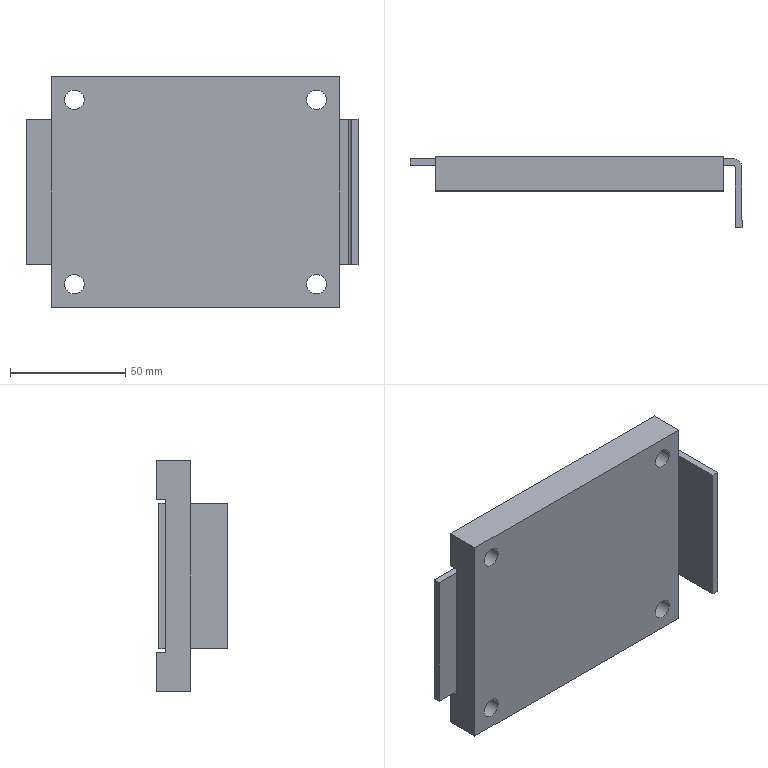Part | SolidWorks | features BaseBody 1, Extrusion 1 | 2 solids | 28 faces | box 144 x 31 x 100 mm | volume 183212 mm3 | plane 18 | cylinder 10 | commonest cylinder face diameters 8.5 x8 2 x1 8 x1
STEP:
#1=CARTESIAN_POINT('',(591.731,149.744,-409.193));
#2=VERTEX_POINT('',#1);
#3=CARTESIAN_POINT('',(587.731,153.744,-409.193));
#4=VERTEX_POINT('',#3);
#5=CARTESIAN_POINT('',(587.731,149.744,-409.193));
#6=DIRECTION('',(0.,0.,1.));
#7=DIRECTION('',(1.,0.,0.));
#8=AXIS2_PLACEMENT_3D('',#5,#6,#7);
#9=CIRCLE('',#8,4.);
#10=EDGE_CURVE('',#2,#4,#9,.T.);
#11=ORIENTED_EDGE('',*,*,#10,.F.);
#12=CARTESIAN_POINT('',(591.731,149.744,-472.193));
#13=VERTEX_POINT('',#12);
#14=CARTESIAN_POINT('',(591.731,149.744,-472.193));
#15=DIRECTION('',(0.,0.,1.));
#16=VECTOR('',#15,1000.);
#17=LINE('',#14,#16);
#18=EDGE_CURVE('',#13,#2,#17,.T.);
#19=ORIENTED_EDGE('',*,*,#18,.F.);
#20=CARTESIAN_POINT('',(587.731,153.744,-472.193));
#21=VERTEX_POINT('',#20);
#22=CARTESIAN_POINT('',(587.731,149.744,-472.193));
#23=DIRECTION('',(0.,0.,1.));
#24=DIRECTION('',(1.,0.,0.));
#25=AXIS2_PLACEMENT_3D('',#22,#23,#24);
#26=CIRCLE('',#25,4.);
#27=EDGE_CURVE('',#13,#21,#26,.T.);
#28=ORIENTED_EDGE('',*,*,#27,.T.);
#29=CARTESIAN_POINT('',(587.731,153.744,-472.193));
#30=DIRECTION('',(0.,0.,1.));
#31=VECTOR('',#30,1000.);
#32=LINE('',#29,#31);
#33=EDGE_CURVE('',#21,#4,#32,.T.);
#34=ORIENTED_EDGE('',*,*,#33,.T.);
#35=EDGE_LOOP('',(#11,#19,#28,#34));
#36=FACE_OUTER_BOUND('',#35,.T.);
#37=CARTESIAN_POINT('',(587.731,149.744,-472.193));
#38=DIRECTION('',(0.,0.,1.));
#39=DIRECTION('',(1.,0.,0.));
#40=AXIS2_PLACEMENT_3D('',#37,#38,#39);
#41=CYLINDRICAL_SURFACE('',#40,4.);
#42=ADVANCED_FACE('',(#36),#41,.T.);
#43=CARTESIAN_POINT('',(591.731,123.744,-409.193));
#44=VERTEX_POINT('',#43);
#45=CARTESIAN_POINT('',(591.731,123.744,-409.193));
#46=DIRECTION('',(0.,1.,0.));
#47=VECTOR('',#46,1000.);
#48=LINE('',#45,#47);
#49=EDGE_CURVE('',#44,#2,#48,.T.);
#50=ORIENTED_EDGE('',*,*,#49,.F.);
#51=CARTESIAN_POINT('',(591.731,123.744,-472.193));
#52=VERTEX_POINT('',#51);
#53=CARTESIAN_POINT('',(591.731,123.744,-472.193));
#54=DIRECTION('',(0.,0.,1.));
#55=VECTOR('',#54,1000.);
#56=LINE('',#53,#55);
#57=EDGE_CURVE('',#52,#44,#56,.T.);
#58=ORIENTED_EDGE('',*,*,#57,.F.);
#59=CARTESIAN_POINT('',(591.731,123.744,-472.193));
#60=DIRECTION('',(0.,1.,0.));
#61=VECTOR('',#60,1000.);
#62=LINE('',#59,#61);
#63=EDGE_CURVE('',#52,#13,#62,.T.);
#64=ORIENTED_EDGE('',*,*,#63,.T.);
#65=ORIENTED_EDGE('',*,*,#18,.T.);
#66=EDGE_LOOP('',(#50,#58,#64,#65));
#67=FACE_OUTER_BOUND('',#66,.T.);
#68=CARTESIAN_POINT('',(591.731,123.744,-472.193));
#69=DIRECTION('',(1.,0.,0.));
#70=DIRECTION('',(0.,1.,0.));
#71=AXIS2_PLACEMENT_3D('',#68,#69,#70);
#72=PLANE('',#71);
#73=ADVANCED_FACE('',(#67),#72,.T.);
#74=CARTESIAN_POINT('',(588.731,123.744,-409.193));
#75=VERTEX_POINT('',#74);
#76=CARTESIAN_POINT('',(588.731,123.744,-409.193));
#77=DIRECTION('',(1.,0.,0.));
#78=VECTOR('',#77,1000.);
#79=LINE('',#76,#78);
#80=EDGE_CURVE('',#75,#44,#79,.T.);
#81=ORIENTED_EDGE('',*,*,#80,.F.);
#82=CARTESIAN_POINT('',(588.731,123.744,-472.193));
#83=VERTEX_POINT('',#82);
#84=CARTESIAN_POINT('',(588.731,123.744,-472.193));
#85=DIRECTION('',(0.,0.,1.));
#86=VECTOR('',#85,1000.);
#87=LINE('',#84,#86);
#88=EDGE_CURVE('',#83,#75,#87,.T.);
#89=ORIENTED_EDGE('',*,*,#88,.F.);
#90=CARTESIAN_POINT('',(588.731,123.744,-472.193));
#91=DIRECTION('',(1.,0.,0.));
#92=VECTOR('',#91,1000.);
#93=LINE('',#90,#92);
#94=EDGE_CURVE('',#83,#52,#93,.T.);
#95=ORIENTED_EDGE('',*,*,#94,.T.);
#96=ORIENTED_EDGE('',*,*,#57,.T.);
#97=EDGE_LOOP('',(#81,#89,#95,#96));
#98=FACE_OUTER_BOUND('',#97,.T.);
#99=CARTESIAN_POINT('',(588.731,123.744,-472.193));
#100=DIRECTION('',(0.,-1.,0.));
#101=DIRECTION('',(1.,0.,0.));
#102=AXIS2_PLACEMENT_3D('',#99,#100,#101);
#103=PLANE('',#102);
#104=ADVANCED_FACE('',(#98),#103,.T.);
#105=CARTESIAN_POINT('',(588.731,149.744,-409.193));
#106=VERTEX_POINT('',#105);
#107=CARTESIAN_POINT('',(588.731,149.744,-409.193));
#108=DIRECTION('',(0.,-1.,0.));
#109=VECTOR('',#108,1000.);
#110=LINE('',#107,#109);
#111=EDGE_CURVE('',#106,#75,#110,.T.);
#112=ORIENTED_EDGE('',*,*,#111,.F.);
#113=CARTESIAN_POINT('',(588.731,149.744,-472.193));
#114=VERTEX_POINT('',#113);
#115=CARTESIAN_POINT('',(588.731,149.744,-472.193));
#116=DIRECTION('',(0.,0.,1.));
#117=VECTOR('',#116,1000.);
#118=LINE('',#115,#117);
#119=EDGE_CURVE('',#114,#106,#118,.T.);
#120=ORIENTED_EDGE('',*,*,#119,.F.);
#121=CARTESIAN_POINT('',(588.731,149.744,-472.193));
#122=DIRECTION('',(0.,-1.,0.));
#123=VECTOR('',#122,1000.);
#124=LINE('',#121,#123);
#125=EDGE_CURVE('',#114,#83,#124,.T.);
#126=ORIENTED_EDGE('',*,*,#125,.T.);
#127=ORIENTED_EDGE('',*,*,#88,.T.);
#128=EDGE_LOOP('',(#112,#120,#126,#127));
#129=FACE_OUTER_BOUND('',#128,.T.);
#130=CARTESIAN_POINT('',(588.731,149.744,-472.193));
#131=DIRECTION('',(-1.,0.,0.));
#132=DIRECTION('',(0.,-1.,0.));
#133=AXIS2_PLACEMENT_3D('',#130,#131,#132);
#134=PLANE('',#133);
#135=ADVANCED_FACE('',(#129),#134,.T.);
#136=CARTESIAN_POINT('',(587.731,150.744,-409.193));
#137=VERTEX_POINT('',#136);
#138=CARTESIAN_POINT('',(587.731,149.744,-409.193));
#139=DIRECTION('',(0.,0.,-1.));
#140=DIRECTION('',(-1.,0.,0.));
#141=AXIS2_PLACEMENT_3D('',#138,#139,#140);
#142=CIRCLE('',#141,1.);
#143=EDGE_CURVE('',#137,#106,#142,.T.);
#144=ORIENTED_EDGE('',*,*,#143,.F.);
#145=CARTESIAN_POINT('',(587.731,150.744,-472.193));
#146=VERTEX_POINT('',#145);
#147=CARTESIAN_POINT('',(587.731,150.744,-472.193));
#148=DIRECTION('',(0.,0.,1.));
#149=VECTOR('',#148,1000.);
#150=LINE('',#147,#149);
#151=EDGE_CURVE('',#146,#137,#150,.T.);
#152=ORIENTED_EDGE('',*,*,#151,.F.);
#153=CARTESIAN_POINT('',(587.731,149.744,-472.193));
#154=DIRECTION('',(0.,0.,-1.));
#155=DIRECTION('',(-1.,0.,0.));
#156=AXIS2_PLACEMENT_3D('',#153,#154,#155);
#157=CIRCLE('',#156,1.);
#158=EDGE_CURVE('',#146,#114,#157,.T.);
#159=ORIENTED_EDGE('',*,*,#158,.T.);
#160=ORIENTED_EDGE('',*,*,#119,.T.);
#161=EDGE_LOOP('',(#144,#152,#159,#160));
#162=FACE_OUTER_BOUND('',#161,.T.);
#163=CARTESIAN_POINT('',(587.731,149.744,-472.193));
#164=DIRECTION('',(0.,0.,1.));
#165=DIRECTION('',(1.,0.,0.));
#166=AXIS2_PLACEMENT_3D('',#163,#164,#165);
#167=CYLINDRICAL_SURFACE('',#166,1.);
#168=ADVANCED_FACE('',(#162),#167,.F.);
#169=CARTESIAN_POINT('',(447.731,150.744,-409.193));
#170=VERTEX_POINT('',#169);
#171=CARTESIAN_POINT('',(447.731,150.744,-409.193));
#172=DIRECTION('',(1.,0.,0.));
#173=VECTOR('',#172,1000.);
#174=LINE('',#171,#173);
#175=EDGE_CURVE('',#170,#137,#174,.T.);
#176=ORIENTED_EDGE('',*,*,#175,.F.);
#177=CARTESIAN_POINT('',(447.731,150.744,-472.193));
#178=VERTEX_POINT('',#177);
#179=CARTESIAN_POINT('',(447.731,150.744,-472.193));
#180=DIRECTION('',(0.,0.,1.));
#181=VECTOR('',#180,1000.);
#182=LINE('',#179,#181);
#183=EDGE_CURVE('',#178,#170,#182,.T.);
#184=ORIENTED_EDGE('',*,*,#183,.F.);
#185=CARTESIAN_POINT('',(447.731,150.744,-472.193));
#186=DIRECTION('',(1.,0.,0.));
#187=VECTOR('',#186,1000.);
#188=LINE('',#185,#187);
#189=EDGE_CURVE('',#178,#146,#188,.T.);
#190=ORIENTED_EDGE('',*,*,#189,.T.);
#191=ORIENTED_EDGE('',*,*,#151,.T.);
#192=EDGE_LOOP('',(#176,#184,#190,#191));
#193=FACE_OUTER_BOUND('',#192,.T.);
#194=CARTESIAN_POINT('',(447.731,150.744,-472.193));
#195=DIRECTION('',(0.,-1.,0.));
#196=DIRECTION('',(0.,0.,-1.));
#197=AXIS2_PLACEMENT_3D('',#194,#195,#196);
#198=PLANE('',#197);
#199=ADVANCED_FACE('',(#193),#198,.T.);
#200=CARTESIAN_POINT('',(447.731,153.744,-409.193));
#201=VERTEX_POINT('',#200);
#202=CARTESIAN_POINT('',(447.731,153.744,-409.193));
#203=DIRECTION('',(0.,-1.,0.));
#204=VECTOR('',#203,1000.);
#205=LINE('',#202,#204);
#206=EDGE_CURVE('',#201,#170,#205,.T.);
#207=ORIENTED_EDGE('',*,*,#206,.F.);
#208=CARTESIAN_POINT('',(447.731,153.744,-472.193));
#209=VERTEX_POINT('',#208);
#210=CARTESIAN_POINT('',(447.731,153.744,-472.193));
#211=DIRECTION('',(0.,0.,1.));
#212=VECTOR('',#211,1000.);
#213=LINE('',#210,#212);
#214=EDGE_CURVE('',#209,#201,#213,.T.);
#215=ORIENTED_EDGE('',*,*,#214,.F.);
#216=CARTESIAN_POINT('',(447.731,153.744,-472.193));
#217=DIRECTION('',(0.,-1.,0.));
#218=VECTOR('',#217,1000.);
#219=LINE('',#216,#218);
#220=EDGE_CURVE('',#209,#178,#219,.T.);
#221=ORIENTED_EDGE('',*,*,#220,.T.);
#222=ORIENTED_EDGE('',*,*,#183,.T.);
#223=EDGE_LOOP('',(#207,#215,#221,#222));
#224=FACE_OUTER_BOUND('',#223,.T.);
#225=CARTESIAN_POINT('',(447.731,153.744,-472.193));
#226=DIRECTION('',(-1.,0.,0.));
#227=DIRECTION('',(0.,0.,1.));
#228=AXIS2_PLACEMENT_3D('',#225,#226,#227);
#229=PLANE('',#228);
#230=ADVANCED_FACE('',(#224),#229,.T.);
#231=CARTESIAN_POINT('',(587.731,153.744,-409.193));
#232=DIRECTION('',(-1.,0.,0.));
#233=VECTOR('',#232,1000.);
#234=LINE('',#231,#233);
#235=EDGE_CURVE('',#4,#201,#234,.T.);
#236=ORIENTED_EDGE('',*,*,#235,.F.);
#237=ORIENTED_EDGE('',*,*,#33,.F.);
#238=CARTESIAN_POINT('',(587.731,153.744,-472.193));
#239=DIRECTION('',(-1.,0.,0.));
#240=VECTOR('',#239,1000.);
#241=LINE('',#238,#240);
#242=EDGE_CURVE('',#21,#209,#241,.T.);
#243=ORIENTED_EDGE('',*,*,#242,.T.);
#244=ORIENTED_EDGE('',*,*,#214,.T.);
#245=EDGE_LOOP('',(#236,#237,#243,#244));
#246=FACE_OUTER_BOUND('',#245,.T.);
#247=CARTESIAN_POINT('',(587.731,153.744,-472.193));
#248=DIRECTION('',(0.,1.,0.));
#249=DIRECTION('',(0.,0.,1.));
#250=AXIS2_PLACEMENT_3D('',#247,#248,#249);
#251=PLANE('',#250);
#252=ADVANCED_FACE('',(#246),#251,.T.);
#253=ORIENTED_EDGE('',*,*,#27,.F.);
#254=ORIENTED_EDGE('',*,*,#63,.F.);
#255=ORIENTED_EDGE('',*,*,#94,.F.);
#256=ORIENTED_EDGE('',*,*,#125,.F.);
#257=ORIENTED_EDGE('',*,*,#158,.F.);
#258=ORIENTED_EDGE('',*,*,#189,.F.);
#259=ORIENTED_EDGE('',*,*,#220,.F.);
#260=ORIENTED_EDGE('',*,*,#242,.F.);
#261=EDGE_LOOP('',(#253,#254,#255,#256,#257,#258,#259,#260));
#262=FACE_OUTER_BOUND('',#261,.T.);
#263=CARTESIAN_POINT('',(587.731,149.744,-472.193));
#264=DIRECTION('',(0.,0.,1.));
#265=DIRECTION('',(1.,0.,0.));
#266=AXIS2_PLACEMENT_3D('',#263,#264,#265);
#267=PLANE('',#266);
#268=ADVANCED_FACE('',(#262),#267,.F.);
#269=ORIENTED_EDGE('',*,*,#10,.T.);
#270=ORIENTED_EDGE('',*,*,#235,.T.);
#271=ORIENTED_EDGE('',*,*,#206,.T.);
#272=ORIENTED_EDGE('',*,*,#175,.T.);
#273=ORIENTED_EDGE('',*,*,#143,.T.);
#274=ORIENTED_EDGE('',*,*,#111,.T.);
#275=ORIENTED_EDGE('',*,*,#80,.T.);
#276=ORIENTED_EDGE('',*,*,#49,.T.);
#277=EDGE_LOOP('',(#269,#270,#271,#272,#273,#274,#275,#276));
#278=FACE_OUTER_BOUND('',#277,.T.);
#279=CARTESIAN_POINT('',(587.731,149.744,-409.193));
#280=DIRECTION('',(0.,0.,1.));
#281=DIRECTION('',(1.,0.,0.));
#282=AXIS2_PLACEMENT_3D('',#279,#280,#281);
#283=PLANE('',#282);
#284=ADVANCED_FACE('',(#278),#283,.T.);
#285=CLOSED_SHELL('',(#42,#73,#104,#135,#168,#199,#230,#252,#268,#284));
#286=MANIFOLD_SOLID_BREP('',#285);
#287=CARTESIAN_POINT('',(569.481,154.744,-480.693));
#288=VERTEX_POINT('',#287);
#289=CARTESIAN_POINT('',(577.981,154.744,-480.693));
#290=VERTEX_POINT('',#289);
#291=CARTESIAN_POINT('',(573.731,154.744,-480.693));
#292=DIRECTION('',(0.,1.,0.));
#293=DIRECTION('',(1.,0.,0.));
#294=AXIS2_PLACEMENT_3D('',#291,#292,#293);
#295=CIRCLE('',#294,4.25);
#296=EDGE_CURVE('',#288,#290,#295,.T.);
#297=ORIENTED_EDGE('',*,*,#296,.T.);
#298=CARTESIAN_POINT('',(577.981,139.744,-480.693));
#299=VERTEX_POINT('',#298);
#300=CARTESIAN_POINT('',(577.981,169.744,-480.693));
#301=DIRECTION('',(0.,-1.,0.));
#302=VECTOR('',#301,1000.);
#303=LINE('',#300,#302);
#304=EDGE_CURVE('',#290,#299,#303,.T.);
#305=ORIENTED_EDGE('',*,*,#304,.T.);
#306=CARTESIAN_POINT('',(569.481,139.744,-480.693));
#307=VERTEX_POINT('',#306);
#308=CARTESIAN_POINT('',(573.731,139.744,-480.693));
#309=DIRECTION('',(0.,-1.,0.));
#310=DIRECTION('',(1.,0.,0.));
#311=AXIS2_PLACEMENT_3D('',#308,#309,#310);
#312=CIRCLE('',#311,4.25);
#313=EDGE_CURVE('',#299,#307,#312,.T.);
#314=ORIENTED_EDGE('',*,*,#313,.T.);
#315=CARTESIAN_POINT('',(569.481,169.744,-480.693));
#316=DIRECTION('',(0.,-1.,0.));
#317=VECTOR('',#316,1000.);
#318=LINE('',#315,#317);
#319=EDGE_CURVE('',#288,#307,#318,.T.);
#320=ORIENTED_EDGE('',*,*,#319,.F.);
#321=EDGE_LOOP('',(#297,#305,#314,#320));
#322=FACE_OUTER_BOUND('',#321,.T.);
#323=CARTESIAN_POINT('',(573.731,169.744,-480.693));
#324=DIRECTION('',(0.,-1.,0.));
#325=DIRECTION('',(-1.,0.,0.));
#326=AXIS2_PLACEMENT_3D('',#323,#324,#325);
#327=CYLINDRICAL_SURFACE('',#326,4.25);
#328=ADVANCED_FACE('',(#322),#327,.F.);
#329=CARTESIAN_POINT('',(464.481,154.744,-400.693));
#330=VERTEX_POINT('',#329);
#331=CARTESIAN_POINT('',(472.981,154.744,-400.693));
#332=VERTEX_POINT('',#331);
#333=CARTESIAN_POINT('',(468.731,154.744,-400.693));
#334=DIRECTION('',(0.,1.,0.));
#335=DIRECTION('',(1.,0.,0.));
#336=AXIS2_PLACEMENT_3D('',#333,#334,#335);
#337=CIRCLE('',#336,4.25);
#338=EDGE_CURVE('',#330,#332,#337,.T.);
#339=ORIENTED_EDGE('',*,*,#338,.T.);
#340=CARTESIAN_POINT('',(472.981,139.744,-400.693));
#341=VERTEX_POINT('',#340);
#342=CARTESIAN_POINT('',(472.981,169.744,-400.693));
#343=DIRECTION('',(0.,-1.,0.));
#344=VECTOR('',#343,1000.);
#345=LINE('',#342,#344);
#346=EDGE_CURVE('',#332,#341,#345,.T.);
#347=ORIENTED_EDGE('',*,*,#346,.T.);
#348=CARTESIAN_POINT('',(464.481,139.744,-400.693));
#349=VERTEX_POINT('',#348);
#350=CARTESIAN_POINT('',(468.731,139.744,-400.693));
#351=DIRECTION('',(0.,-1.,0.));
#352=DIRECTION('',(1.,0.,0.));
#353=AXIS2_PLACEMENT_3D('',#350,#351,#352);
#354=CIRCLE('',#353,4.25);
#355=EDGE_CURVE('',#341,#349,#354,.T.);
#356=ORIENTED_EDGE('',*,*,#355,.T.);
#357=CARTESIAN_POINT('',(464.481,169.744,-400.693));
#358=DIRECTION('',(0.,-1.,0.));
#359=VECTOR('',#358,1000.);
#360=LINE('',#357,#359);
#361=EDGE_CURVE('',#330,#349,#360,.T.);
#362=ORIENTED_EDGE('',*,*,#361,.F.);
#363=EDGE_LOOP('',(#339,#347,#356,#362));
#364=FACE_OUTER_BOUND('',#363,.T.);
#365=CARTESIAN_POINT('',(468.731,169.744,-400.693));
#366=DIRECTION('',(0.,-1.,0.));
#367=DIRECTION('',(-1.,0.,0.));
#368=AXIS2_PLACEMENT_3D('',#365,#366,#367);
#369=CYLINDRICAL_SURFACE('',#368,4.25);
#370=ADVANCED_FACE('',(#364),#369,.F.);
#371=CARTESIAN_POINT('',(464.481,154.744,-480.693));
#372=VERTEX_POINT('',#371);
#373=CARTESIAN_POINT('',(472.981,154.744,-480.693));
#374=VERTEX_POINT('',#373);
#375=CARTESIAN_POINT('',(468.731,154.744,-480.693));
#376=DIRECTION('',(0.,1.,0.));
#377=DIRECTION('',(1.,0.,0.));
#378=AXIS2_PLACEMENT_3D('',#375,#376,#377);
#379=CIRCLE('',#378,4.25);
#380=EDGE_CURVE('',#372,#374,#379,.T.);
#381=ORIENTED_EDGE('',*,*,#380,.T.);
#382=CARTESIAN_POINT('',(472.981,139.744,-480.693));
#383=VERTEX_POINT('',#382);
#384=CARTESIAN_POINT('',(472.981,169.744,-480.693));
#385=DIRECTION('',(0.,-1.,0.));
#386=VECTOR('',#385,1000.);
#387=LINE('',#384,#386);
#388=EDGE_CURVE('',#374,#383,#387,.T.);
#389=ORIENTED_EDGE('',*,*,#388,.T.);
#390=CARTESIAN_POINT('',(464.481,139.744,-480.693));
#391=VERTEX_POINT('',#390);
#392=CARTESIAN_POINT('',(468.731,139.744,-480.693));
#393=DIRECTION('',(0.,-1.,0.));
#394=DIRECTION('',(-1.,0.,0.));
#395=AXIS2_PLACEMENT_3D('',#392,#393,#394);
#396=CIRCLE('',#395,4.25);
#397=EDGE_CURVE('',#383,#391,#396,.T.);
#398=ORIENTED_EDGE('',*,*,#397,.T.);
#399=CARTESIAN_POINT('',(464.481,169.744,-480.693));
#400=DIRECTION('',(0.,-1.,0.));
#401=VECTOR('',#400,1000.);
#402=LINE('',#399,#401);
#403=EDGE_CURVE('',#372,#391,#402,.T.);
#404=ORIENTED_EDGE('',*,*,#403,.F.);
#405=EDGE_LOOP('',(#381,#389,#398,#404));
#406=FACE_OUTER_BOUND('',#405,.T.);
#407=CARTESIAN_POINT('',(468.731,169.744,-480.693));
#408=DIRECTION('',(0.,-1.,0.));
#409=DIRECTION('',(-1.,0.,0.));
#410=AXIS2_PLACEMENT_3D('',#407,#408,#409);
#411=CYLINDRICAL_SURFACE('',#410,4.25);
#412=ADVANCED_FACE('',(#406),#411,.F.);
#413=CARTESIAN_POINT('',(569.481,154.744,-400.693));
#414=VERTEX_POINT('',#413);
#415=CARTESIAN_POINT('',(577.981,154.744,-400.693));
#416=VERTEX_POINT('',#415);
#417=CARTESIAN_POINT('',(573.731,154.744,-400.693));
#418=DIRECTION('',(0.,1.,0.));
#419=DIRECTION('',(1.,0.,0.));
#420=AXIS2_PLACEMENT_3D('',#417,#418,#419);
#421=CIRCLE('',#420,4.25);
#422=EDGE_CURVE('',#414,#416,#421,.T.);
#423=ORIENTED_EDGE('',*,*,#422,.T.);
#424=CARTESIAN_POINT('',(577.981,139.744,-400.693));
#425=VERTEX_POINT('',#424);
#426=CARTESIAN_POINT('',(577.981,169.744,-400.693));
#427=DIRECTION('',(0.,-1.,0.));
#428=VECTOR('',#427,1000.);
#429=LINE('',#426,#428);
#430=EDGE_CURVE('',#416,#425,#429,.T.);
#431=ORIENTED_EDGE('',*,*,#430,.T.);
#432=CARTESIAN_POINT('',(569.481,139.744,-400.693));
#433=VERTEX_POINT('',#432);
#434=CARTESIAN_POINT('',(573.731,139.744,-400.693));
#435=DIRECTION('',(0.,-1.,0.));
#436=DIRECTION('',(-1.,0.,0.));
#437=AXIS2_PLACEMENT_3D('',#434,#435,#436);
#438=CIRCLE('',#437,4.25);
#439=EDGE_CURVE('',#425,#433,#438,.T.);
#440=ORIENTED_EDGE('',*,*,#439,.T.);
#441=CARTESIAN_POINT('',(569.481,169.744,-400.693));
#442=DIRECTION('',(0.,-1.,0.));
#443=VECTOR('',#442,1000.);
#444=LINE('',#441,#443);
#445=EDGE_CURVE('',#414,#433,#444,.T.);
#446=ORIENTED_EDGE('',*,*,#445,.F.);
#447=EDGE_LOOP('',(#423,#431,#440,#446));
#448=FACE_OUTER_BOUND('',#447,.T.);
#449=CARTESIAN_POINT('',(573.731,169.744,-400.693));
#450=DIRECTION('',(0.,-1.,0.));
#451=DIRECTION('',(-1.,0.,0.));
#452=AXIS2_PLACEMENT_3D('',#449,#450,#451);
#453=CYLINDRICAL_SURFACE('',#452,4.25);
#454=ADVANCED_FACE('',(#448),#453,.F.);
#455=CARTESIAN_POINT('',(458.731,154.744,-407.693));
#456=VERTEX_POINT('',#455);
#457=CARTESIAN_POINT('',(583.731,154.744,-407.693));
#458=VERTEX_POINT('',#457);
#459=CARTESIAN_POINT('',(521.231,154.744,-407.693));
#460=DIRECTION('',(1.,0.,0.));
#461=VECTOR('',#460,1000.);
#462=LINE('',#459,#461);
#463=EDGE_CURVE('',#456,#458,#462,.T.);
#464=ORIENTED_EDGE('',*,*,#463,.F.);
#465=CARTESIAN_POINT('',(458.731,154.744,-390.693));
#466=VERTEX_POINT('',#465);
#467=CARTESIAN_POINT('',(458.731,154.744,-390.693));
#468=DIRECTION('',(0.,0.,-1.));
#469=VECTOR('',#468,1000.);
#470=LINE('',#467,#469);
#471=EDGE_CURVE('',#466,#456,#470,.T.);
#472=ORIENTED_EDGE('',*,*,#471,.F.);
#473=CARTESIAN_POINT('',(583.731,154.744,-390.693));
#474=VERTEX_POINT('',#473);
#475=CARTESIAN_POINT('',(583.731,154.744,-390.693));
#476=DIRECTION('',(-1.,0.,0.));
#477=VECTOR('',#476,1000.);
#478=LINE('',#475,#477);
#479=EDGE_CURVE('',#474,#466,#478,.T.);
#480=ORIENTED_EDGE('',*,*,#479,.F.);
#481=CARTESIAN_POINT('',(583.731,154.744,-390.693));
#482=DIRECTION('',(0.,0.,1.));
#483=VECTOR('',#482,1000.);
#484=LINE('',#481,#483);
#485=EDGE_CURVE('',#458,#474,#484,.T.);
#486=ORIENTED_EDGE('',*,*,#485,.F.);
#487=EDGE_LOOP('',(#464,#472,#480,#486));
#488=FACE_OUTER_BOUND('',#487,.T.);
#489=ORIENTED_EDGE('',*,*,#422,.F.);
#490=CARTESIAN_POINT('',(573.731,154.744,-400.693));
#491=DIRECTION('',(0.,1.,0.));
#492=DIRECTION('',(1.,0.,0.));
#493=AXIS2_PLACEMENT_3D('',#490,#491,#492);
#494=CIRCLE('',#493,4.25);
#495=EDGE_CURVE('',#416,#414,#494,.T.);
#496=ORIENTED_EDGE('',*,*,#495,.F.);
#497=EDGE_LOOP('',(#489,#496));
#498=FACE_BOUND('',#497,.T.);
#499=ORIENTED_EDGE('',*,*,#338,.F.);
#500=CARTESIAN_POINT('',(468.731,154.744,-400.693));
#501=DIRECTION('',(0.,1.,0.));
#502=DIRECTION('',(1.,0.,0.));
#503=AXIS2_PLACEMENT_3D('',#500,#501,#502);
#504=CIRCLE('',#503,4.25);
#505=EDGE_CURVE('',#332,#330,#504,.T.);
#506=ORIENTED_EDGE('',*,*,#505,.F.);
#507=EDGE_LOOP('',(#499,#506));
#508=FACE_BOUND('',#507,.T.);
#509=CARTESIAN_POINT('',(521.231,154.744,-440.693));
#510=DIRECTION('',(0.,1.,0.));
#511=DIRECTION('',(1.,0.,0.));
#512=AXIS2_PLACEMENT_3D('',#509,#510,#511);
#513=PLANE('',#512);
#514=ADVANCED_FACE('',(#488,#498,#508),#513,.T.);
#515=ORIENTED_EDGE('',*,*,#471,.T.);
#516=CARTESIAN_POINT('',(458.731,150.744,-407.693));
#517=VERTEX_POINT('',#516);
#518=CARTESIAN_POINT('',(458.731,139.744,-407.693));
#519=DIRECTION('',(0.,-1.,0.));
#520=VECTOR('',#519,1000.);
#521=LINE('',#518,#520);
#522=EDGE_CURVE('',#456,#517,#521,.T.);
#523=ORIENTED_EDGE('',*,*,#522,.T.);
#524=CARTESIAN_POINT('',(458.731,150.744,-473.693));
#525=VERTEX_POINT('',#524);
#526=CARTESIAN_POINT('',(458.731,150.744,-390.693));
#527=DIRECTION('',(0.,0.,-1.));
#528=VECTOR('',#527,1000.);
#529=LINE('',#526,#528);
#530=EDGE_CURVE('',#517,#525,#529,.T.);
#531=ORIENTED_EDGE('',*,*,#530,.T.);
#532=CARTESIAN_POINT('',(458.731,154.744,-473.693));
#533=VERTEX_POINT('',#532);
#534=CARTESIAN_POINT('',(458.731,139.744,-473.693));
#535=DIRECTION('',(0.,1.,0.));
#536=VECTOR('',#535,1000.);
#537=LINE('',#534,#536);
#538=EDGE_CURVE('',#525,#533,#537,.T.);
#539=ORIENTED_EDGE('',*,*,#538,.T.);
#540=CARTESIAN_POINT('',(458.731,154.744,-490.693));
#541=VERTEX_POINT('',#540);
#542=CARTESIAN_POINT('',(458.731,154.744,-390.693));
#543=DIRECTION('',(0.,0.,-1.));
#544=VECTOR('',#543,1000.);
#545=LINE('',#542,#544);
#546=EDGE_CURVE('',#533,#541,#545,.T.);
#547=ORIENTED_EDGE('',*,*,#546,.T.);
#548=CARTESIAN_POINT('',(458.731,139.744,-490.693));
#549=VERTEX_POINT('',#548);
#550=CARTESIAN_POINT('',(458.731,139.744,-490.693));
#551=DIRECTION('',(0.,1.,0.));
#552=VECTOR('',#551,1000.);
#553=LINE('',#550,#552);
#554=EDGE_CURVE('',#549,#541,#553,.T.);
#555=ORIENTED_EDGE('',*,*,#554,.F.);
#556=CARTESIAN_POINT('',(458.731,139.744,-390.693));
#557=VERTEX_POINT('',#556);
#558=CARTESIAN_POINT('',(458.731,139.744,-390.693));
#559=DIRECTION('',(0.,0.,-1.));
#560=VECTOR('',#559,1000.);
#561=LINE('',#558,#560);
#562=EDGE_CURVE('',#557,#549,#561,.T.);
#563=ORIENTED_EDGE('',*,*,#562,.F.);
#564=CARTESIAN_POINT('',(458.731,139.744,-390.693));
#565=DIRECTION('',(0.,1.,0.));
#566=VECTOR('',#565,1000.);
#567=LINE('',#564,#566);
#568=EDGE_CURVE('',#557,#466,#567,.T.);
#569=ORIENTED_EDGE('',*,*,#568,.T.);
#570=EDGE_LOOP('',(#515,#523,#531,#539,#547,#555,#563,#569));
#571=FACE_OUTER_BOUND('',#570,.T.);
#572=CARTESIAN_POINT('',(458.731,139.744,-390.693));
#573=DIRECTION('',(1.,0.,0.));
#574=DIRECTION('',(0.,-1.,0.));
#575=AXIS2_PLACEMENT_3D('',#572,#573,#574);
#576=PLANE('',#575);
#577=ADVANCED_FACE('',(#571),#576,.F.);
#578=CARTESIAN_POINT('',(583.731,154.744,-490.693));
#579=VERTEX_POINT('',#578);
#580=CARTESIAN_POINT('',(583.731,154.744,-490.693));
#581=DIRECTION('',(1.,0.,0.));
#582=VECTOR('',#581,1000.);
#583=LINE('',#580,#582);
#584=EDGE_CURVE('',#541,#579,#583,.T.);
#585=ORIENTED_EDGE('',*,*,#584,.T.);
#586=CARTESIAN_POINT('',(583.731,139.744,-490.693));
#587=VERTEX_POINT('',#586);
#588=CARTESIAN_POINT('',(583.731,139.744,-490.693));
#589=DIRECTION('',(0.,1.,0.));
#590=VECTOR('',#589,1000.);
#591=LINE('',#588,#590);
#592=EDGE_CURVE('',#587,#579,#591,.T.);
#593=ORIENTED_EDGE('',*,*,#592,.F.);
#594=CARTESIAN_POINT('',(583.731,139.744,-490.693));
#595=DIRECTION('',(1.,0.,0.));
#596=VECTOR('',#595,1000.);
#597=LINE('',#594,#596);
#598=EDGE_CURVE('',#549,#587,#597,.T.);
#599=ORIENTED_EDGE('',*,*,#598,.F.);
#600=ORIENTED_EDGE('',*,*,#554,.T.);
#601=EDGE_LOOP('',(#585,#593,#599,#600));
#602=FACE_OUTER_BOUND('',#601,.T.);
#603=CARTESIAN_POINT('',(583.731,139.744,-490.693));
#604=DIRECTION('',(0.,0.,1.));
#605=DIRECTION('',(0.,1.,0.));
#606=AXIS2_PLACEMENT_3D('',#603,#604,#605);
#607=PLANE('',#606);
#608=ADVANCED_FACE('',(#602),#607,.F.);
#609=CARTESIAN_POINT('',(583.731,150.744,-407.693));
#610=VERTEX_POINT('',#609);
#611=CARTESIAN_POINT('',(583.731,150.744,-473.693));
#612=VERTEX_POINT('',#611);
#613=CARTESIAN_POINT('',(583.731,150.744,-407.693));
#614=DIRECTION('',(0.,0.,-1.));
#615=VECTOR('',#614,1000.);
#616=LINE('',#613,#615);
#617=EDGE_CURVE('',#610,#612,#616,.T.);
#618=ORIENTED_EDGE('',*,*,#617,.F.);
#619=CARTESIAN_POINT('',(583.731,186.186,-407.693));
#620=DIRECTION('',(0.,-1.,0.));
#621=VECTOR('',#620,1000.);
#622=LINE('',#619,#621);
#623=EDGE_CURVE('',#458,#610,#622,.T.);
#624=ORIENTED_EDGE('',*,*,#623,.F.);
#625=ORIENTED_EDGE('',*,*,#485,.T.);
#626=CARTESIAN_POINT('',(583.731,139.744,-390.693));
#627=VERTEX_POINT('',#626);
#628=CARTESIAN_POINT('',(583.731,139.744,-390.693));
#629=DIRECTION('',(0.,1.,0.));
#630=VECTOR('',#629,1000.);
#631=LINE('',#628,#630);
#632=EDGE_CURVE('',#627,#474,#631,.T.);
#633=ORIENTED_EDGE('',*,*,#632,.F.);
#634=CARTESIAN_POINT('',(583.731,139.744,-390.693));
#635=DIRECTION('',(0.,0.,1.));
#636=VECTOR('',#635,1000.);
#637=LINE('',#634,#636);
#638=EDGE_CURVE('',#587,#627,#637,.T.);
#639=ORIENTED_EDGE('',*,*,#638,.F.);
#640=ORIENTED_EDGE('',*,*,#592,.T.);
#641=CARTESIAN_POINT('',(583.731,154.744,-473.693));
#642=VERTEX_POINT('',#641);
#643=CARTESIAN_POINT('',(583.731,154.744,-390.693));
#644=DIRECTION('',(0.,0.,1.));
#645=VECTOR('',#644,1000.);
#646=LINE('',#643,#645);
#647=EDGE_CURVE('',#579,#642,#646,.T.);
#648=ORIENTED_EDGE('',*,*,#647,.T.);
#649=CARTESIAN_POINT('',(583.731,186.186,-473.693));
#650=DIRECTION('',(0.,1.,0.));
#651=VECTOR('',#650,1000.);
#652=LINE('',#649,#651);
#653=EDGE_CURVE('',#612,#642,#652,.T.);
#654=ORIENTED_EDGE('',*,*,#653,.F.);
#655=EDGE_LOOP('',(#618,#624,#625,#633,#639,#640,#648,#654));
#656=FACE_OUTER_BOUND('',#655,.T.);
#657=CARTESIAN_POINT('',(583.731,139.744,-390.693));
#658=DIRECTION('',(-1.,0.,0.));
#659=DIRECTION('',(0.,1.,0.));
#660=AXIS2_PLACEMENT_3D('',#657,#658,#659);
#661=PLANE('',#660);
#662=ADVANCED_FACE('',(#656),#661,.F.);
#663=ORIENTED_EDGE('',*,*,#479,.T.);
#664=ORIENTED_EDGE('',*,*,#568,.F.);
#665=CARTESIAN_POINT('',(583.731,139.744,-390.693));
#666=DIRECTION('',(-1.,0.,0.));
#667=VECTOR('',#666,1000.);
#668=LINE('',#665,#667);
#669=EDGE_CURVE('',#627,#557,#668,.T.);
#670=ORIENTED_EDGE('',*,*,#669,.F.);
#671=ORIENTED_EDGE('',*,*,#632,.T.);
#672=EDGE_LOOP('',(#663,#664,#670,#671));
#673=FACE_OUTER_BOUND('',#672,.T.);
#674=CARTESIAN_POINT('',(583.731,139.744,-390.693));
#675=DIRECTION('',(0.,0.,-1.));
#676=DIRECTION('',(0.,-1.,0.));
#677=AXIS2_PLACEMENT_3D('',#674,#675,#676);
#678=PLANE('',#677);
#679=ADVANCED_FACE('',(#673),#678,.F.);
#680=CARTESIAN_POINT('',(573.731,139.744,-480.693));
#681=DIRECTION('',(0.,-1.,0.));
#682=DIRECTION('',(1.,0.,0.));
#683=AXIS2_PLACEMENT_3D('',#680,#681,#682);
#684=CIRCLE('',#683,4.25);
#685=EDGE_CURVE('',#307,#299,#684,.T.);
#686=ORIENTED_EDGE('',*,*,#685,.F.);
#687=ORIENTED_EDGE('',*,*,#313,.F.);
#688=EDGE_LOOP('',(#686,#687));
#689=FACE_BOUND('',#688,.T.);
#690=CARTESIAN_POINT('',(468.731,139.744,-400.693));
#691=DIRECTION('',(0.,-1.,0.));
#692=DIRECTION('',(1.,0.,0.));
#693=AXIS2_PLACEMENT_3D('',#690,#691,#692);
#694=CIRCLE('',#693,4.25);
#695=EDGE_CURVE('',#349,#341,#694,.T.);
#696=ORIENTED_EDGE('',*,*,#695,.F.);
#697=ORIENTED_EDGE('',*,*,#355,.F.);
#698=EDGE_LOOP('',(#696,#697));
#699=FACE_BOUND('',#698,.T.);
#700=CARTESIAN_POINT('',(468.731,139.744,-480.693));
#701=DIRECTION('',(0.,-1.,0.));
#702=DIRECTION('',(-1.,0.,0.));
#703=AXIS2_PLACEMENT_3D('',#700,#701,#702);
#704=CIRCLE('',#703,4.25);
#705=EDGE_CURVE('',#391,#383,#704,.T.);
#706=ORIENTED_EDGE('',*,*,#705,.F.);
#707=ORIENTED_EDGE('',*,*,#397,.F.);
#708=EDGE_LOOP('',(#706,#707));
#709=FACE_BOUND('',#708,.T.);
#710=CARTESIAN_POINT('',(573.731,139.744,-400.693));
#711=DIRECTION('',(0.,-1.,0.));
#712=DIRECTION('',(-1.,0.,0.));
#713=AXIS2_PLACEMENT_3D('',#710,#711,#712);
#714=CIRCLE('',#713,4.25);
#715=EDGE_CURVE('',#433,#425,#714,.T.);
#716=ORIENTED_EDGE('',*,*,#715,.F.);
#717=ORIENTED_EDGE('',*,*,#439,.F.);
#718=EDGE_LOOP('',(#716,#717));
#719=FACE_BOUND('',#718,.T.);
#720=ORIENTED_EDGE('',*,*,#562,.T.);
#721=ORIENTED_EDGE('',*,*,#598,.T.);
#722=ORIENTED_EDGE('',*,*,#638,.T.);
#723=ORIENTED_EDGE('',*,*,#669,.T.);
#724=EDGE_LOOP('',(#720,#721,#722,#723));
#725=FACE_OUTER_BOUND('',#724,.T.);
#726=CARTESIAN_POINT('',(521.231,139.744,-440.693));
#727=DIRECTION('',(0.,1.,0.));
#728=DIRECTION('',(1.,0.,0.));
#729=AXIS2_PLACEMENT_3D('',#726,#727,#728);
#730=PLANE('',#729);
#731=ADVANCED_FACE('',(#689,#699,#709,#719,#725),#730,.F.);
#732=CARTESIAN_POINT('',(521.231,154.744,-473.693));
#733=DIRECTION('',(-1.,0.,0.));
#734=VECTOR('',#733,1000.);
#735=LINE('',#732,#734);
#736=EDGE_CURVE('',#642,#533,#735,.T.);
#737=ORIENTED_EDGE('',*,*,#736,.F.);
#738=ORIENTED_EDGE('',*,*,#647,.F.);
#739=ORIENTED_EDGE('',*,*,#584,.F.);
#740=ORIENTED_EDGE('',*,*,#546,.F.);
#741=EDGE_LOOP('',(#737,#738,#739,#740));
#742=FACE_OUTER_BOUND('',#741,.T.);
#743=ORIENTED_EDGE('',*,*,#296,.F.);
#744=CARTESIAN_POINT('',(573.731,154.744,-480.693));
#745=DIRECTION('',(0.,1.,0.));
#746=DIRECTION('',(1.,0.,0.));
#747=AXIS2_PLACEMENT_3D('',#744,#745,#746);
#748=CIRCLE('',#747,4.25);
#749=EDGE_CURVE('',#290,#288,#748,.T.);
#750=ORIENTED_EDGE('',*,*,#749,.F.);
#751=EDGE_LOOP('',(#743,#750));
#752=FACE_BOUND('',#751,.T.);
#753=ORIENTED_EDGE('',*,*,#380,.F.);
#754=CARTESIAN_POINT('',(468.731,154.744,-480.693));
#755=DIRECTION('',(0.,1.,0.));
#756=DIRECTION('',(1.,0.,0.));
#757=AXIS2_PLACEMENT_3D('',#754,#755,#756);
#758=CIRCLE('',#757,4.25);
#759=EDGE_CURVE('',#374,#372,#758,.T.);
#760=ORIENTED_EDGE('',*,*,#759,.F.);
#761=EDGE_LOOP('',(#753,#760));
#762=FACE_BOUND('',#761,.T.);
#763=CARTESIAN_POINT('',(521.231,154.744,-440.693));
#764=DIRECTION('',(0.,1.,0.));
#765=DIRECTION('',(1.,0.,0.));
#766=AXIS2_PLACEMENT_3D('',#763,#764,#765);
#767=PLANE('',#766);
#768=ADVANCED_FACE('',(#742,#752,#762),#767,.T.);
#769=ORIENTED_EDGE('',*,*,#430,.F.);
#770=ORIENTED_EDGE('',*,*,#495,.T.);
#771=ORIENTED_EDGE('',*,*,#445,.T.);
#772=ORIENTED_EDGE('',*,*,#715,.T.);
#773=EDGE_LOOP('',(#769,#770,#771,#772));
#774=FACE_OUTER_BOUND('',#773,.T.);
#775=CARTESIAN_POINT('',(573.731,169.744,-400.693));
#776=DIRECTION('',(0.,-1.,0.));
#777=DIRECTION('',(-1.,0.,0.));
#778=AXIS2_PLACEMENT_3D('',#775,#776,#777);
#779=CYLINDRICAL_SURFACE('',#778,4.25);
#780=ADVANCED_FACE('',(#774),#779,.F.);
#781=ORIENTED_EDGE('',*,*,#388,.F.);
#782=ORIENTED_EDGE('',*,*,#759,.T.);
#783=ORIENTED_EDGE('',*,*,#403,.T.);
#784=ORIENTED_EDGE('',*,*,#705,.T.);
#785=EDGE_LOOP('',(#781,#782,#783,#784));
#786=FACE_OUTER_BOUND('',#785,.T.);
#787=CARTESIAN_POINT('',(468.731,169.744,-480.693));
#788=DIRECTION('',(0.,-1.,0.));
#789=DIRECTION('',(-1.,0.,0.));
#790=AXIS2_PLACEMENT_3D('',#787,#788,#789);
#791=CYLINDRICAL_SURFACE('',#790,4.25);
#792=ADVANCED_FACE('',(#786),#791,.F.);
#793=ORIENTED_EDGE('',*,*,#346,.F.);
#794=ORIENTED_EDGE('',*,*,#505,.T.);
#795=ORIENTED_EDGE('',*,*,#361,.T.);
#796=ORIENTED_EDGE('',*,*,#695,.T.);
#797=EDGE_LOOP('',(#793,#794,#795,#796));
#798=FACE_OUTER_BOUND('',#797,.T.);
#799=CARTESIAN_POINT('',(468.731,169.744,-400.693));
#800=DIRECTION('',(0.,-1.,0.));
#801=DIRECTION('',(-1.,0.,0.));
#802=AXIS2_PLACEMENT_3D('',#799,#800,#801);
#803=CYLINDRICAL_SURFACE('',#802,4.25);
#804=ADVANCED_FACE('',(#798),#803,.F.);
#805=ORIENTED_EDGE('',*,*,#304,.F.);
#806=ORIENTED_EDGE('',*,*,#749,.T.);
#807=ORIENTED_EDGE('',*,*,#319,.T.);
#808=ORIENTED_EDGE('',*,*,#685,.T.);
#809=EDGE_LOOP('',(#805,#806,#807,#808));
#810=FACE_OUTER_BOUND('',#809,.T.);
#811=CARTESIAN_POINT('',(573.731,169.744,-480.693));
#812=DIRECTION('',(0.,-1.,0.));
#813=DIRECTION('',(-1.,0.,0.));
#814=AXIS2_PLACEMENT_3D('',#811,#812,#813);
#815=CYLINDRICAL_SURFACE('',#814,4.25);
#816=ADVANCED_FACE('',(#810),#815,.F.);
#817=CARTESIAN_POINT('',(283.731,150.744,-407.693));
#818=DIRECTION('',(1.,0.,0.));
#819=VECTOR('',#818,1000.);
#820=LINE('',#817,#819);
#821=EDGE_CURVE('',#517,#610,#820,.T.);
#822=ORIENTED_EDGE('',*,*,#821,.T.);
#823=ORIENTED_EDGE('',*,*,#617,.T.);
#824=CARTESIAN_POINT('',(283.731,150.744,-473.693));
#825=DIRECTION('',(1.,0.,0.));
#826=VECTOR('',#825,1000.);
#827=LINE('',#824,#826);
#828=EDGE_CURVE('',#525,#612,#827,.T.);
#829=ORIENTED_EDGE('',*,*,#828,.F.);
#830=ORIENTED_EDGE('',*,*,#530,.F.);
#831=EDGE_LOOP('',(#822,#823,#829,#830));
#832=FACE_OUTER_BOUND('',#831,.T.);
#833=CARTESIAN_POINT('',(283.731,150.744,-407.693));
#834=DIRECTION('',(0.,-1.,0.));
#835=DIRECTION('',(0.,0.,1.));
#836=AXIS2_PLACEMENT_3D('',#833,#834,#835);
#837=PLANE('',#836);
#838=ADVANCED_FACE('',(#832),#837,.F.);
#839=ORIENTED_EDGE('',*,*,#463,.T.);
#840=ORIENTED_EDGE('',*,*,#623,.T.);
#841=ORIENTED_EDGE('',*,*,#821,.F.);
#842=ORIENTED_EDGE('',*,*,#522,.F.);
#843=EDGE_LOOP('',(#839,#840,#841,#842));
#844=FACE_OUTER_BOUND('',#843,.T.);
#845=CARTESIAN_POINT('',(283.731,186.186,-407.693));
#846=DIRECTION('',(0.,0.,1.));
#847=DIRECTION('',(0.,1.,0.));
#848=AXIS2_PLACEMENT_3D('',#845,#846,#847);
#849=PLANE('',#848);
#850=ADVANCED_FACE('',(#844),#849,.F.);
#851=ORIENTED_EDGE('',*,*,#828,.T.);
#852=ORIENTED_EDGE('',*,*,#653,.T.);
#853=ORIENTED_EDGE('',*,*,#736,.T.);
#854=ORIENTED_EDGE('',*,*,#538,.F.);
#855=EDGE_LOOP('',(#851,#852,#853,#854));
#856=FACE_OUTER_BOUND('',#855,.T.);
#857=CARTESIAN_POINT('',(283.731,186.186,-473.693));
#858=DIRECTION('',(0.,0.,-1.));
#859=DIRECTION('',(0.,-1.,0.));
#860=AXIS2_PLACEMENT_3D('',#857,#858,#859);
#861=PLANE('',#860);
#862=ADVANCED_FACE('',(#856),#861,.F.);
#863=CLOSED_SHELL('',(#328,#370,#412,#454,#514,#577,#608,#662,#679,#731,#768,#780,#792,#804,#816,#838,#850,#862));
#864=MANIFOLD_SOLID_BREP('',#863);
#865=CARTESIAN_POINT('',(0.,0.,0.));
#866=DIRECTION('',(0.,0.,1.));
#867=DIRECTION('',(1.,0.,0.));
#868=AXIS2_PLACEMENT_3D('',#865,#866,#867);
#869=(LENGTH_UNIT()NAMED_UNIT(*)SI_UNIT(.MILLI.,.METRE.));
#870=UNCERTAINTY_MEASURE_WITH_UNIT(LENGTH_MEASURE(0.00001),#869,'','');
#871=(NAMED_UNIT(*)PLANE_ANGLE_UNIT()SI_UNIT($,.RADIAN.));
#872=(NAMED_UNIT(*)SI_UNIT($,.STERADIAN.)SOLID_ANGLE_UNIT());
#873=(GEOMETRIC_REPRESENTATION_CONTEXT(3)GLOBAL_UNCERTAINTY_ASSIGNED_CONTEXT((#870))GLOBAL_UNIT_ASSIGNED_CONTEXT((#869,#871,#872))REPRESENTATION_CONTEXT('',''));
#874=ADVANCED_BREP_SHAPE_REPRESENTATION('',(#286,#864,#868),#873);